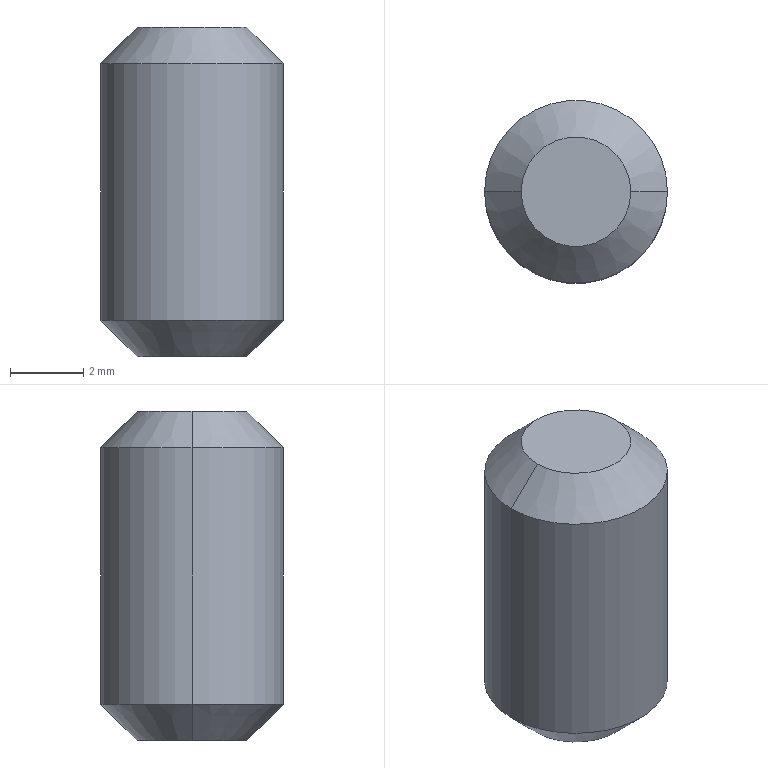Part | SolidWorks | features Chamfer 1, Extrusion 1 | 1 solid | 8 faces | box 5 x 5 x 9 mm | volume 163.101 mm3 | cone 4 | cylinder 2 | plane 2 | commonest cylinder face diameters 5 x2
STEP:
#1=CARTESIAN_POINT('',(1.5,0.,9.));
#2=VERTEX_POINT('',#1);
#3=CARTESIAN_POINT('',(-1.5,0.,9.));
#4=VERTEX_POINT('',#3);
#5=CARTESIAN_POINT('',(0.,0.,9.));
#6=DIRECTION('',(0.,0.,1.));
#7=DIRECTION('',(1.,0.,0.));
#8=AXIS2_PLACEMENT_3D('',#5,#6,#7);
#9=CIRCLE('',#8,1.5);
#10=EDGE_CURVE('',#2,#4,#9,.T.);
#11=ORIENTED_EDGE('',*,*,#10,.F.);
#12=CARTESIAN_POINT('',(2.5,0.,8.));
#13=VERTEX_POINT('',#12);
#14=CARTESIAN_POINT('',(1.5,0.,9.));
#15=DIRECTION('',(0.7071,0.,-0.7071));
#16=VECTOR('',#15,1000.);
#17=LINE('',#14,#16);
#18=EDGE_CURVE('',#2,#13,#17,.T.);
#19=ORIENTED_EDGE('',*,*,#18,.T.);
#20=CARTESIAN_POINT('',(-2.5,0.,8.));
#21=VERTEX_POINT('',#20);
#22=CARTESIAN_POINT('',(0.,0.,8.));
#23=DIRECTION('',(0.,0.,-1.));
#24=DIRECTION('',(1.,0.,0.));
#25=AXIS2_PLACEMENT_3D('',#22,#23,#24);
#26=CIRCLE('',#25,2.5);
#27=EDGE_CURVE('',#21,#13,#26,.T.);
#28=ORIENTED_EDGE('',*,*,#27,.F.);
#29=CARTESIAN_POINT('',(-1.5,0.,9.));
#30=DIRECTION('',(-0.7071,0.,-0.7071));
#31=VECTOR('',#30,1000.);
#32=LINE('',#29,#31);
#33=EDGE_CURVE('',#4,#21,#32,.T.);
#34=ORIENTED_EDGE('',*,*,#33,.F.);
#35=EDGE_LOOP('',(#11,#19,#28,#34));
#36=FACE_OUTER_BOUND('',#35,.T.);
#37=CARTESIAN_POINT('',(0.,0.,9.));
#38=DIRECTION('',(0.,0.,-1.));
#39=DIRECTION('',(-1.,0.,0.));
#40=AXIS2_PLACEMENT_3D('',#37,#38,#39);
#41=CONICAL_SURFACE('',#40,1.5,0.7854);
#42=ADVANCED_FACE('',(#36),#41,.T.);
#43=CARTESIAN_POINT('',(-1.5,0.,0.));
#44=VERTEX_POINT('',#43);
#45=CARTESIAN_POINT('',(1.5,0.,0.));
#46=VERTEX_POINT('',#45);
#47=CARTESIAN_POINT('',(0.,0.,0.));
#48=DIRECTION('',(0.,0.,-1.));
#49=DIRECTION('',(1.,0.,0.));
#50=AXIS2_PLACEMENT_3D('',#47,#48,#49);
#51=CIRCLE('',#50,1.5);
#52=EDGE_CURVE('',#44,#46,#51,.T.);
#53=ORIENTED_EDGE('',*,*,#52,.F.);
#54=CARTESIAN_POINT('',(-2.5,0.,1.));
#55=VERTEX_POINT('',#54);
#56=CARTESIAN_POINT('',(-2.5,0.,1.));
#57=DIRECTION('',(-0.7071,0.,0.7071));
#58=VECTOR('',#57,1000.);
#59=LINE('',#56,#58);
#60=EDGE_CURVE('',#44,#55,#59,.T.);
#61=ORIENTED_EDGE('',*,*,#60,.T.);
#62=CARTESIAN_POINT('',(2.5,0.,1.));
#63=VERTEX_POINT('',#62);
#64=CARTESIAN_POINT('',(0.,0.,1.));
#65=DIRECTION('',(0.,0.,1.));
#66=DIRECTION('',(1.,0.,0.));
#67=AXIS2_PLACEMENT_3D('',#64,#65,#66);
#68=CIRCLE('',#67,2.5);
#69=EDGE_CURVE('',#63,#55,#68,.T.);
#70=ORIENTED_EDGE('',*,*,#69,.F.);
#71=CARTESIAN_POINT('',(2.5,0.,1.));
#72=DIRECTION('',(0.7071,0.,0.7071));
#73=VECTOR('',#72,1000.);
#74=LINE('',#71,#73);
#75=EDGE_CURVE('',#46,#63,#74,.T.);
#76=ORIENTED_EDGE('',*,*,#75,.F.);
#77=EDGE_LOOP('',(#53,#61,#70,#76));
#78=FACE_OUTER_BOUND('',#77,.T.);
#79=CARTESIAN_POINT('',(0.,0.,1.));
#80=DIRECTION('',(0.,0.,1.));
#81=DIRECTION('',(1.,0.,0.));
#82=AXIS2_PLACEMENT_3D('',#79,#80,#81);
#83=CONICAL_SURFACE('',#82,2.5,0.7854);
#84=ADVANCED_FACE('',(#78),#83,.T.);
#85=ORIENTED_EDGE('',*,*,#27,.T.);
#86=CARTESIAN_POINT('',(2.5,0.,9.));
#87=DIRECTION('',(0.,0.,-1.));
#88=VECTOR('',#87,1000.);
#89=LINE('',#86,#88);
#90=EDGE_CURVE('',#13,#63,#89,.T.);
#91=ORIENTED_EDGE('',*,*,#90,.T.);
#92=ORIENTED_EDGE('',*,*,#69,.T.);
#93=CARTESIAN_POINT('',(-2.5,0.,9.));
#94=DIRECTION('',(0.,0.,-1.));
#95=VECTOR('',#94,1000.);
#96=LINE('',#93,#95);
#97=EDGE_CURVE('',#21,#55,#96,.T.);
#98=ORIENTED_EDGE('',*,*,#97,.F.);
#99=EDGE_LOOP('',(#85,#91,#92,#98));
#100=FACE_OUTER_BOUND('',#99,.T.);
#101=CARTESIAN_POINT('',(0.,0.,9.));
#102=DIRECTION('',(0.,0.,-1.));
#103=DIRECTION('',(-1.,0.,0.));
#104=AXIS2_PLACEMENT_3D('',#101,#102,#103);
#105=CYLINDRICAL_SURFACE('',#104,2.5);
#106=ADVANCED_FACE('',(#100),#105,.T.);
#107=ORIENTED_EDGE('',*,*,#90,.F.);
#108=CARTESIAN_POINT('',(0.,0.,8.));
#109=DIRECTION('',(0.,0.,-1.));
#110=DIRECTION('',(1.,0.,0.));
#111=AXIS2_PLACEMENT_3D('',#108,#109,#110);
#112=CIRCLE('',#111,2.5);
#113=EDGE_CURVE('',#13,#21,#112,.T.);
#114=ORIENTED_EDGE('',*,*,#113,.T.);
#115=ORIENTED_EDGE('',*,*,#97,.T.);
#116=CARTESIAN_POINT('',(0.,0.,1.));
#117=DIRECTION('',(0.,0.,1.));
#118=DIRECTION('',(1.,0.,0.));
#119=AXIS2_PLACEMENT_3D('',#116,#117,#118);
#120=CIRCLE('',#119,2.5);
#121=EDGE_CURVE('',#55,#63,#120,.T.);
#122=ORIENTED_EDGE('',*,*,#121,.T.);
#123=EDGE_LOOP('',(#107,#114,#115,#122));
#124=FACE_OUTER_BOUND('',#123,.T.);
#125=CARTESIAN_POINT('',(0.,0.,9.));
#126=DIRECTION('',(0.,0.,-1.));
#127=DIRECTION('',(-1.,0.,0.));
#128=AXIS2_PLACEMENT_3D('',#125,#126,#127);
#129=CYLINDRICAL_SURFACE('',#128,2.5);
#130=ADVANCED_FACE('',(#124),#129,.T.);
#131=CARTESIAN_POINT('',(0.,0.,9.));
#132=DIRECTION('',(0.,0.,1.));
#133=DIRECTION('',(1.,0.,0.));
#134=AXIS2_PLACEMENT_3D('',#131,#132,#133);
#135=CIRCLE('',#134,1.5);
#136=EDGE_CURVE('',#4,#2,#135,.T.);
#137=ORIENTED_EDGE('',*,*,#136,.T.);
#138=ORIENTED_EDGE('',*,*,#10,.T.);
#139=EDGE_LOOP('',(#137,#138));
#140=FACE_OUTER_BOUND('',#139,.T.);
#141=CARTESIAN_POINT('',(0.,0.,9.));
#142=DIRECTION('',(0.,0.,1.));
#143=DIRECTION('',(1.,0.,0.));
#144=AXIS2_PLACEMENT_3D('',#141,#142,#143);
#145=PLANE('',#144);
#146=ADVANCED_FACE('',(#140),#145,.T.);
#147=CARTESIAN_POINT('',(0.,0.,0.));
#148=DIRECTION('',(0.,0.,-1.));
#149=DIRECTION('',(1.,0.,0.));
#150=AXIS2_PLACEMENT_3D('',#147,#148,#149);
#151=CIRCLE('',#150,1.5);
#152=EDGE_CURVE('',#46,#44,#151,.T.);
#153=ORIENTED_EDGE('',*,*,#152,.T.);
#154=ORIENTED_EDGE('',*,*,#52,.T.);
#155=EDGE_LOOP('',(#153,#154));
#156=FACE_OUTER_BOUND('',#155,.T.);
#157=CARTESIAN_POINT('',(0.,0.,0.));
#158=DIRECTION('',(0.,0.,1.));
#159=DIRECTION('',(1.,0.,0.));
#160=AXIS2_PLACEMENT_3D('',#157,#158,#159);
#161=PLANE('',#160);
#162=ADVANCED_FACE('',(#156),#161,.F.);
#163=ORIENTED_EDGE('',*,*,#60,.F.);
#164=ORIENTED_EDGE('',*,*,#152,.F.);
#165=ORIENTED_EDGE('',*,*,#75,.T.);
#166=ORIENTED_EDGE('',*,*,#121,.F.);
#167=EDGE_LOOP('',(#163,#164,#165,#166));
#168=FACE_OUTER_BOUND('',#167,.T.);
#169=CARTESIAN_POINT('',(0.,0.,1.));
#170=DIRECTION('',(0.,0.,1.));
#171=DIRECTION('',(1.,0.,0.));
#172=AXIS2_PLACEMENT_3D('',#169,#170,#171);
#173=CONICAL_SURFACE('',#172,2.5,0.7854);
#174=ADVANCED_FACE('',(#168),#173,.T.);
#175=ORIENTED_EDGE('',*,*,#18,.F.);
#176=ORIENTED_EDGE('',*,*,#136,.F.);
#177=ORIENTED_EDGE('',*,*,#33,.T.);
#178=ORIENTED_EDGE('',*,*,#113,.F.);
#179=EDGE_LOOP('',(#175,#176,#177,#178));
#180=FACE_OUTER_BOUND('',#179,.T.);
#181=CARTESIAN_POINT('',(0.,0.,9.));
#182=DIRECTION('',(0.,0.,-1.));
#183=DIRECTION('',(-1.,0.,0.));
#184=AXIS2_PLACEMENT_3D('',#181,#182,#183);
#185=CONICAL_SURFACE('',#184,1.5,0.7854);
#186=ADVANCED_FACE('',(#180),#185,.T.);
#187=CLOSED_SHELL('',(#42,#84,#106,#130,#146,#162,#174,#186));
#188=MANIFOLD_SOLID_BREP('',#187);
#189=CARTESIAN_POINT('',(0.,0.,0.));
#190=DIRECTION('',(0.,0.,1.));
#191=DIRECTION('',(1.,0.,0.));
#192=AXIS2_PLACEMENT_3D('',#189,#190,#191);
#193=(LENGTH_UNIT()NAMED_UNIT(*)SI_UNIT(.MILLI.,.METRE.));
#194=UNCERTAINTY_MEASURE_WITH_UNIT(LENGTH_MEASURE(0.00001),#193,'','');
#195=(NAMED_UNIT(*)PLANE_ANGLE_UNIT()SI_UNIT($,.RADIAN.));
#196=(NAMED_UNIT(*)SI_UNIT($,.STERADIAN.)SOLID_ANGLE_UNIT());
#197=(GEOMETRIC_REPRESENTATION_CONTEXT(3)GLOBAL_UNCERTAINTY_ASSIGNED_CONTEXT((#194))GLOBAL_UNIT_ASSIGNED_CONTEXT((#193,#195,#196))REPRESENTATION_CONTEXT('',''));
#198=ADVANCED_BREP_SHAPE_REPRESENTATION('',(#188,#192),#197);